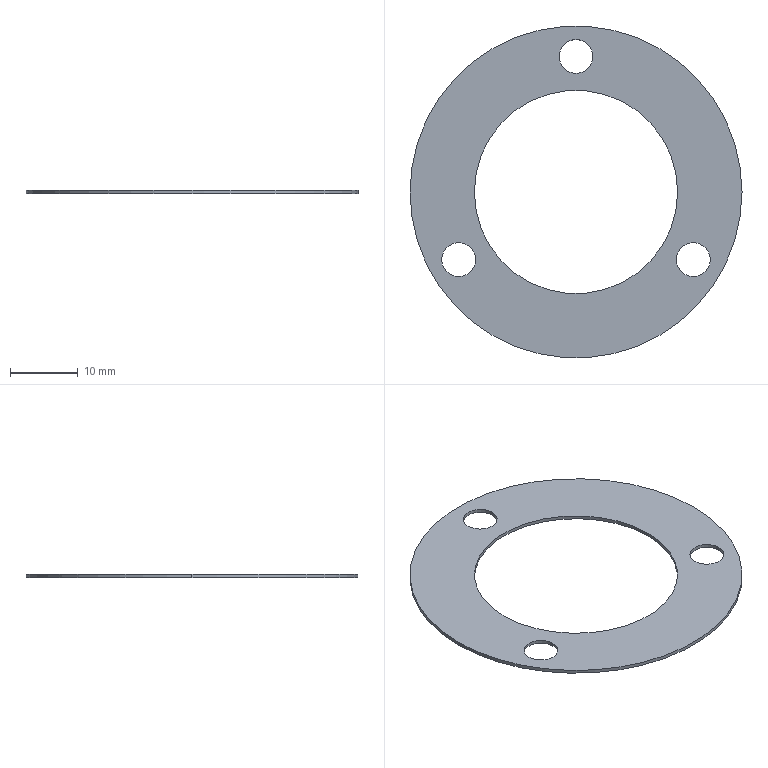Part | SolidWorks | features Extrusion 1, ICE 1 | 1 solid | 12 faces | box 49 x 49 x 0.5 mm | volume 559.989 mm3 | cylinder 10 | plane 2 | commonest cylinder face diameters 5 x6 30 x2 49 x2
STEP:
#1=CARTESIAN_POINT('',(-2.5,20.,0.));
#2=VERTEX_POINT('',#1);
#3=CARTESIAN_POINT('',(2.5,20.,0.));
#4=VERTEX_POINT('',#3);
#5=CARTESIAN_POINT('',(0.,20.,0.));
#6=DIRECTION('',(0.,0.,1.));
#7=DIRECTION('',(1.,0.,0.));
#8=AXIS2_PLACEMENT_3D('',#5,#6,#7);
#9=CIRCLE('',#8,2.5);
#10=EDGE_CURVE('',#2,#4,#9,.T.);
#11=ORIENTED_EDGE('',*,*,#10,.F.);
#12=CARTESIAN_POINT('',(-2.5,20.,0.5));
#13=VERTEX_POINT('',#12);
#14=CARTESIAN_POINT('',(-2.5,20.,0.));
#15=DIRECTION('',(0.,0.,1.));
#16=VECTOR('',#15,1000.);
#17=LINE('',#14,#16);
#18=EDGE_CURVE('',#2,#13,#17,.T.);
#19=ORIENTED_EDGE('',*,*,#18,.T.);
#20=CARTESIAN_POINT('',(2.5,20.,0.5));
#21=VERTEX_POINT('',#20);
#22=CARTESIAN_POINT('',(0.,20.,0.5));
#23=DIRECTION('',(0.,0.,1.));
#24=DIRECTION('',(1.,0.,0.));
#25=AXIS2_PLACEMENT_3D('',#22,#23,#24);
#26=CIRCLE('',#25,2.5);
#27=EDGE_CURVE('',#13,#21,#26,.T.);
#28=ORIENTED_EDGE('',*,*,#27,.T.);
#29=CARTESIAN_POINT('',(2.5,20.,0.));
#30=DIRECTION('',(0.,0.,1.));
#31=VECTOR('',#30,1000.);
#32=LINE('',#29,#31);
#33=EDGE_CURVE('',#4,#21,#32,.T.);
#34=ORIENTED_EDGE('',*,*,#33,.F.);
#35=EDGE_LOOP('',(#11,#19,#28,#34));
#36=FACE_OUTER_BOUND('',#35,.T.);
#37=CARTESIAN_POINT('',(0.,20.,0.));
#38=DIRECTION('',(0.,0.,1.));
#39=DIRECTION('',(1.,0.,0.));
#40=AXIS2_PLACEMENT_3D('',#37,#38,#39);
#41=CYLINDRICAL_SURFACE('',#40,2.5);
#42=ADVANCED_FACE('',(#36),#41,.F.);
#43=CARTESIAN_POINT('',(14.821,-10.,0.));
#44=VERTEX_POINT('',#43);
#45=CARTESIAN_POINT('',(19.821,-10.,0.));
#46=VERTEX_POINT('',#45);
#47=CARTESIAN_POINT('',(17.321,-10.,0.));
#48=DIRECTION('',(0.,0.,1.));
#49=DIRECTION('',(1.,0.,0.));
#50=AXIS2_PLACEMENT_3D('',#47,#48,#49);
#51=CIRCLE('',#50,2.5);
#52=EDGE_CURVE('',#44,#46,#51,.T.);
#53=ORIENTED_EDGE('',*,*,#52,.F.);
#54=CARTESIAN_POINT('',(14.821,-10.,0.5));
#55=VERTEX_POINT('',#54);
#56=CARTESIAN_POINT('',(14.821,-10.,0.));
#57=DIRECTION('',(0.,0.,1.));
#58=VECTOR('',#57,1000.);
#59=LINE('',#56,#58);
#60=EDGE_CURVE('',#44,#55,#59,.T.);
#61=ORIENTED_EDGE('',*,*,#60,.T.);
#62=CARTESIAN_POINT('',(19.821,-10.,0.5));
#63=VERTEX_POINT('',#62);
#64=CARTESIAN_POINT('',(17.321,-10.,0.5));
#65=DIRECTION('',(0.,0.,1.));
#66=DIRECTION('',(1.,0.,0.));
#67=AXIS2_PLACEMENT_3D('',#64,#65,#66);
#68=CIRCLE('',#67,2.5);
#69=EDGE_CURVE('',#55,#63,#68,.T.);
#70=ORIENTED_EDGE('',*,*,#69,.T.);
#71=CARTESIAN_POINT('',(19.821,-10.,0.));
#72=DIRECTION('',(0.,0.,1.));
#73=VECTOR('',#72,1000.);
#74=LINE('',#71,#73);
#75=EDGE_CURVE('',#46,#63,#74,.T.);
#76=ORIENTED_EDGE('',*,*,#75,.F.);
#77=EDGE_LOOP('',(#53,#61,#70,#76));
#78=FACE_OUTER_BOUND('',#77,.T.);
#79=CARTESIAN_POINT('',(17.321,-10.,0.));
#80=DIRECTION('',(0.,0.,1.));
#81=DIRECTION('',(1.,0.,0.));
#82=AXIS2_PLACEMENT_3D('',#79,#80,#81);
#83=CYLINDRICAL_SURFACE('',#82,2.5);
#84=ADVANCED_FACE('',(#78),#83,.F.);
#85=CARTESIAN_POINT('',(-19.821,-10.,0.));
#86=VERTEX_POINT('',#85);
#87=CARTESIAN_POINT('',(-14.821,-10.,0.));
#88=VERTEX_POINT('',#87);
#89=CARTESIAN_POINT('',(-17.321,-10.,0.));
#90=DIRECTION('',(0.,0.,1.));
#91=DIRECTION('',(1.,0.,0.));
#92=AXIS2_PLACEMENT_3D('',#89,#90,#91);
#93=CIRCLE('',#92,2.5);
#94=EDGE_CURVE('',#86,#88,#93,.T.);
#95=ORIENTED_EDGE('',*,*,#94,.F.);
#96=CARTESIAN_POINT('',(-19.821,-10.,0.5));
#97=VERTEX_POINT('',#96);
#98=CARTESIAN_POINT('',(-19.821,-10.,0.));
#99=DIRECTION('',(0.,0.,1.));
#100=VECTOR('',#99,1000.);
#101=LINE('',#98,#100);
#102=EDGE_CURVE('',#86,#97,#101,.T.);
#103=ORIENTED_EDGE('',*,*,#102,.T.);
#104=CARTESIAN_POINT('',(-14.821,-10.,0.5));
#105=VERTEX_POINT('',#104);
#106=CARTESIAN_POINT('',(-17.321,-10.,0.5));
#107=DIRECTION('',(0.,0.,1.));
#108=DIRECTION('',(1.,0.,0.));
#109=AXIS2_PLACEMENT_3D('',#106,#107,#108);
#110=CIRCLE('',#109,2.5);
#111=EDGE_CURVE('',#97,#105,#110,.T.);
#112=ORIENTED_EDGE('',*,*,#111,.T.);
#113=CARTESIAN_POINT('',(-14.821,-10.,0.));
#114=DIRECTION('',(0.,0.,1.));
#115=VECTOR('',#114,1000.);
#116=LINE('',#113,#115);
#117=EDGE_CURVE('',#88,#105,#116,.T.);
#118=ORIENTED_EDGE('',*,*,#117,.F.);
#119=EDGE_LOOP('',(#95,#103,#112,#118));
#120=FACE_OUTER_BOUND('',#119,.T.);
#121=CARTESIAN_POINT('',(-17.321,-10.,0.));
#122=DIRECTION('',(0.,0.,1.));
#123=DIRECTION('',(1.,0.,0.));
#124=AXIS2_PLACEMENT_3D('',#121,#122,#123);
#125=CYLINDRICAL_SURFACE('',#124,2.5);
#126=ADVANCED_FACE('',(#120),#125,.F.);
#127=CARTESIAN_POINT('',(-15.,0.,0.5));
#128=VERTEX_POINT('',#127);
#129=CARTESIAN_POINT('',(15.,0.,0.5));
#130=VERTEX_POINT('',#129);
#131=CARTESIAN_POINT('',(0.,0.,0.5));
#132=DIRECTION('',(0.,0.,1.));
#133=DIRECTION('',(1.,0.,0.));
#134=AXIS2_PLACEMENT_3D('',#131,#132,#133);
#135=CIRCLE('',#134,15.);
#136=EDGE_CURVE('',#128,#130,#135,.T.);
#137=ORIENTED_EDGE('',*,*,#136,.T.);
#138=CARTESIAN_POINT('',(15.,0.,0.));
#139=VERTEX_POINT('',#138);
#140=CARTESIAN_POINT('',(15.,0.,0.5));
#141=DIRECTION('',(0.,0.,-1.));
#142=VECTOR('',#141,1000.);
#143=LINE('',#140,#142);
#144=EDGE_CURVE('',#130,#139,#143,.T.);
#145=ORIENTED_EDGE('',*,*,#144,.T.);
#146=CARTESIAN_POINT('',(-15.,0.,0.));
#147=VERTEX_POINT('',#146);
#148=CARTESIAN_POINT('',(0.,0.,0.));
#149=DIRECTION('',(0.,0.,1.));
#150=DIRECTION('',(1.,0.,0.));
#151=AXIS2_PLACEMENT_3D('',#148,#149,#150);
#152=CIRCLE('',#151,15.);
#153=EDGE_CURVE('',#147,#139,#152,.T.);
#154=ORIENTED_EDGE('',*,*,#153,.F.);
#155=CARTESIAN_POINT('',(-15.,0.,0.5));
#156=DIRECTION('',(0.,0.,-1.));
#157=VECTOR('',#156,1000.);
#158=LINE('',#155,#157);
#159=EDGE_CURVE('',#128,#147,#158,.T.);
#160=ORIENTED_EDGE('',*,*,#159,.F.);
#161=EDGE_LOOP('',(#137,#145,#154,#160));
#162=FACE_OUTER_BOUND('',#161,.T.);
#163=CARTESIAN_POINT('',(0.,0.,0.5));
#164=DIRECTION('',(0.,0.,-1.));
#165=DIRECTION('',(-1.,0.,0.));
#166=AXIS2_PLACEMENT_3D('',#163,#164,#165);
#167=CYLINDRICAL_SURFACE('',#166,15.);
#168=ADVANCED_FACE('',(#162),#167,.F.);
#169=CARTESIAN_POINT('',(24.5,0.,0.5));
#170=VERTEX_POINT('',#169);
#171=CARTESIAN_POINT('',(-24.5,0.,0.5));
#172=VERTEX_POINT('',#171);
#173=CARTESIAN_POINT('',(0.,0.,0.5));
#174=DIRECTION('',(0.,0.,1.));
#175=DIRECTION('',(1.,0.,0.));
#176=AXIS2_PLACEMENT_3D('',#173,#174,#175);
#177=CIRCLE('',#176,24.5);
#178=EDGE_CURVE('',#170,#172,#177,.T.);
#179=ORIENTED_EDGE('',*,*,#178,.F.);
#180=CARTESIAN_POINT('',(24.5,0.,0.));
#181=VERTEX_POINT('',#180);
#182=CARTESIAN_POINT('',(24.5,0.,0.5));
#183=DIRECTION('',(0.,0.,-1.));
#184=VECTOR('',#183,1000.);
#185=LINE('',#182,#184);
#186=EDGE_CURVE('',#170,#181,#185,.T.);
#187=ORIENTED_EDGE('',*,*,#186,.T.);
#188=CARTESIAN_POINT('',(-24.5,0.,0.));
#189=VERTEX_POINT('',#188);
#190=CARTESIAN_POINT('',(0.,0.,0.));
#191=DIRECTION('',(0.,0.,1.));
#192=DIRECTION('',(1.,0.,0.));
#193=AXIS2_PLACEMENT_3D('',#190,#191,#192);
#194=CIRCLE('',#193,24.5);
#195=EDGE_CURVE('',#181,#189,#194,.T.);
#196=ORIENTED_EDGE('',*,*,#195,.T.);
#197=CARTESIAN_POINT('',(-24.5,0.,0.5));
#198=DIRECTION('',(0.,0.,-1.));
#199=VECTOR('',#198,1000.);
#200=LINE('',#197,#199);
#201=EDGE_CURVE('',#172,#189,#200,.T.);
#202=ORIENTED_EDGE('',*,*,#201,.F.);
#203=EDGE_LOOP('',(#179,#187,#196,#202));
#204=FACE_OUTER_BOUND('',#203,.T.);
#205=CARTESIAN_POINT('',(0.,0.,0.5));
#206=DIRECTION('',(0.,0.,-1.));
#207=DIRECTION('',(-1.,0.,0.));
#208=AXIS2_PLACEMENT_3D('',#205,#206,#207);
#209=CYLINDRICAL_SURFACE('',#208,24.5);
#210=ADVANCED_FACE('',(#204),#209,.T.);
#211=CARTESIAN_POINT('',(0.,20.,0.5));
#212=DIRECTION('',(0.,0.,1.));
#213=DIRECTION('',(1.,0.,0.));
#214=AXIS2_PLACEMENT_3D('',#211,#212,#213);
#215=CIRCLE('',#214,2.5);
#216=EDGE_CURVE('',#21,#13,#215,.T.);
#217=ORIENTED_EDGE('',*,*,#216,.F.);
#218=ORIENTED_EDGE('',*,*,#27,.F.);
#219=EDGE_LOOP('',(#217,#218));
#220=FACE_BOUND('',#219,.T.);
#221=CARTESIAN_POINT('',(17.321,-10.,0.5));
#222=DIRECTION('',(0.,0.,1.));
#223=DIRECTION('',(1.,0.,0.));
#224=AXIS2_PLACEMENT_3D('',#221,#222,#223);
#225=CIRCLE('',#224,2.5);
#226=EDGE_CURVE('',#63,#55,#225,.T.);
#227=ORIENTED_EDGE('',*,*,#226,.F.);
#228=ORIENTED_EDGE('',*,*,#69,.F.);
#229=EDGE_LOOP('',(#227,#228));
#230=FACE_BOUND('',#229,.T.);
#231=CARTESIAN_POINT('',(-17.321,-10.,0.5));
#232=DIRECTION('',(0.,0.,1.));
#233=DIRECTION('',(1.,0.,0.));
#234=AXIS2_PLACEMENT_3D('',#231,#232,#233);
#235=CIRCLE('',#234,2.5);
#236=EDGE_CURVE('',#105,#97,#235,.T.);
#237=ORIENTED_EDGE('',*,*,#236,.F.);
#238=ORIENTED_EDGE('',*,*,#111,.F.);
#239=EDGE_LOOP('',(#237,#238));
#240=FACE_BOUND('',#239,.T.);
#241=CARTESIAN_POINT('',(0.,0.,0.5));
#242=DIRECTION('',(0.,0.,1.));
#243=DIRECTION('',(1.,0.,0.));
#244=AXIS2_PLACEMENT_3D('',#241,#242,#243);
#245=CIRCLE('',#244,24.5);
#246=EDGE_CURVE('',#172,#170,#245,.T.);
#247=ORIENTED_EDGE('',*,*,#246,.T.);
#248=ORIENTED_EDGE('',*,*,#178,.T.);
#249=EDGE_LOOP('',(#247,#248));
#250=FACE_OUTER_BOUND('',#249,.T.);
#251=ORIENTED_EDGE('',*,*,#136,.F.);
#252=CARTESIAN_POINT('',(0.,0.,0.5));
#253=DIRECTION('',(0.,0.,1.));
#254=DIRECTION('',(1.,0.,0.));
#255=AXIS2_PLACEMENT_3D('',#252,#253,#254);
#256=CIRCLE('',#255,15.);
#257=EDGE_CURVE('',#130,#128,#256,.T.);
#258=ORIENTED_EDGE('',*,*,#257,.F.);
#259=EDGE_LOOP('',(#251,#258));
#260=FACE_BOUND('',#259,.T.);
#261=CARTESIAN_POINT('',(0.,0.,0.5));
#262=DIRECTION('',(0.,0.,1.));
#263=DIRECTION('',(1.,0.,0.));
#264=AXIS2_PLACEMENT_3D('',#261,#262,#263);
#265=PLANE('',#264);
#266=ADVANCED_FACE('',(#220,#230,#240,#250,#260),#265,.T.);
#267=CARTESIAN_POINT('',(0.,20.,0.));
#268=DIRECTION('',(0.,0.,1.));
#269=DIRECTION('',(1.,0.,0.));
#270=AXIS2_PLACEMENT_3D('',#267,#268,#269);
#271=CIRCLE('',#270,2.5);
#272=EDGE_CURVE('',#4,#2,#271,.T.);
#273=ORIENTED_EDGE('',*,*,#272,.T.);
#274=ORIENTED_EDGE('',*,*,#10,.T.);
#275=EDGE_LOOP('',(#273,#274));
#276=FACE_BOUND('',#275,.T.);
#277=CARTESIAN_POINT('',(17.321,-10.,0.));
#278=DIRECTION('',(0.,0.,1.));
#279=DIRECTION('',(1.,0.,0.));
#280=AXIS2_PLACEMENT_3D('',#277,#278,#279);
#281=CIRCLE('',#280,2.5);
#282=EDGE_CURVE('',#46,#44,#281,.T.);
#283=ORIENTED_EDGE('',*,*,#282,.T.);
#284=ORIENTED_EDGE('',*,*,#52,.T.);
#285=EDGE_LOOP('',(#283,#284));
#286=FACE_BOUND('',#285,.T.);
#287=CARTESIAN_POINT('',(-17.321,-10.,0.));
#288=DIRECTION('',(0.,0.,1.));
#289=DIRECTION('',(1.,0.,0.));
#290=AXIS2_PLACEMENT_3D('',#287,#288,#289);
#291=CIRCLE('',#290,2.5);
#292=EDGE_CURVE('',#88,#86,#291,.T.);
#293=ORIENTED_EDGE('',*,*,#292,.T.);
#294=ORIENTED_EDGE('',*,*,#94,.T.);
#295=EDGE_LOOP('',(#293,#294));
#296=FACE_BOUND('',#295,.T.);
#297=CARTESIAN_POINT('',(0.,0.,0.));
#298=DIRECTION('',(0.,0.,1.));
#299=DIRECTION('',(1.,0.,0.));
#300=AXIS2_PLACEMENT_3D('',#297,#298,#299);
#301=CIRCLE('',#300,24.5);
#302=EDGE_CURVE('',#189,#181,#301,.T.);
#303=ORIENTED_EDGE('',*,*,#302,.F.);
#304=ORIENTED_EDGE('',*,*,#195,.F.);
#305=EDGE_LOOP('',(#303,#304));
#306=FACE_OUTER_BOUND('',#305,.T.);
#307=ORIENTED_EDGE('',*,*,#153,.T.);
#308=CARTESIAN_POINT('',(0.,0.,0.));
#309=DIRECTION('',(0.,0.,1.));
#310=DIRECTION('',(1.,0.,0.));
#311=AXIS2_PLACEMENT_3D('',#308,#309,#310);
#312=CIRCLE('',#311,15.);
#313=EDGE_CURVE('',#139,#147,#312,.T.);
#314=ORIENTED_EDGE('',*,*,#313,.T.);
#315=EDGE_LOOP('',(#307,#314));
#316=FACE_BOUND('',#315,.T.);
#317=CARTESIAN_POINT('',(0.,0.,0.));
#318=DIRECTION('',(0.,0.,1.));
#319=DIRECTION('',(1.,0.,0.));
#320=AXIS2_PLACEMENT_3D('',#317,#318,#319);
#321=PLANE('',#320);
#322=ADVANCED_FACE('',(#276,#286,#296,#306,#316),#321,.F.);
#323=ORIENTED_EDGE('',*,*,#186,.F.);
#324=ORIENTED_EDGE('',*,*,#246,.F.);
#325=ORIENTED_EDGE('',*,*,#201,.T.);
#326=ORIENTED_EDGE('',*,*,#302,.T.);
#327=EDGE_LOOP('',(#323,#324,#325,#326));
#328=FACE_OUTER_BOUND('',#327,.T.);
#329=CARTESIAN_POINT('',(0.,0.,0.5));
#330=DIRECTION('',(0.,0.,-1.));
#331=DIRECTION('',(-1.,0.,0.));
#332=AXIS2_PLACEMENT_3D('',#329,#330,#331);
#333=CYLINDRICAL_SURFACE('',#332,24.5);
#334=ADVANCED_FACE('',(#328),#333,.T.);
#335=ORIENTED_EDGE('',*,*,#144,.F.);
#336=ORIENTED_EDGE('',*,*,#257,.T.);
#337=ORIENTED_EDGE('',*,*,#159,.T.);
#338=ORIENTED_EDGE('',*,*,#313,.F.);
#339=EDGE_LOOP('',(#335,#336,#337,#338));
#340=FACE_OUTER_BOUND('',#339,.T.);
#341=CARTESIAN_POINT('',(0.,0.,0.5));
#342=DIRECTION('',(0.,0.,-1.));
#343=DIRECTION('',(-1.,0.,0.));
#344=AXIS2_PLACEMENT_3D('',#341,#342,#343);
#345=CYLINDRICAL_SURFACE('',#344,15.);
#346=ADVANCED_FACE('',(#340),#345,.F.);
#347=ORIENTED_EDGE('',*,*,#102,.F.);
#348=ORIENTED_EDGE('',*,*,#292,.F.);
#349=ORIENTED_EDGE('',*,*,#117,.T.);
#350=ORIENTED_EDGE('',*,*,#236,.T.);
#351=EDGE_LOOP('',(#347,#348,#349,#350));
#352=FACE_OUTER_BOUND('',#351,.T.);
#353=CARTESIAN_POINT('',(-17.321,-10.,0.));
#354=DIRECTION('',(0.,0.,1.));
#355=DIRECTION('',(1.,0.,0.));
#356=AXIS2_PLACEMENT_3D('',#353,#354,#355);
#357=CYLINDRICAL_SURFACE('',#356,2.5);
#358=ADVANCED_FACE('',(#352),#357,.F.);
#359=ORIENTED_EDGE('',*,*,#60,.F.);
#360=ORIENTED_EDGE('',*,*,#282,.F.);
#361=ORIENTED_EDGE('',*,*,#75,.T.);
#362=ORIENTED_EDGE('',*,*,#226,.T.);
#363=EDGE_LOOP('',(#359,#360,#361,#362));
#364=FACE_OUTER_BOUND('',#363,.T.);
#365=CARTESIAN_POINT('',(17.321,-10.,0.));
#366=DIRECTION('',(0.,0.,1.));
#367=DIRECTION('',(1.,0.,0.));
#368=AXIS2_PLACEMENT_3D('',#365,#366,#367);
#369=CYLINDRICAL_SURFACE('',#368,2.5);
#370=ADVANCED_FACE('',(#364),#369,.F.);
#371=ORIENTED_EDGE('',*,*,#18,.F.);
#372=ORIENTED_EDGE('',*,*,#272,.F.);
#373=ORIENTED_EDGE('',*,*,#33,.T.);
#374=ORIENTED_EDGE('',*,*,#216,.T.);
#375=EDGE_LOOP('',(#371,#372,#373,#374));
#376=FACE_OUTER_BOUND('',#375,.T.);
#377=CARTESIAN_POINT('',(0.,20.,0.));
#378=DIRECTION('',(0.,0.,1.));
#379=DIRECTION('',(1.,0.,0.));
#380=AXIS2_PLACEMENT_3D('',#377,#378,#379);
#381=CYLINDRICAL_SURFACE('',#380,2.5);
#382=ADVANCED_FACE('',(#376),#381,.F.);
#383=CLOSED_SHELL('',(#42,#84,#126,#168,#210,#266,#322,#334,#346,#358,#370,#382));
#384=MANIFOLD_SOLID_BREP('',#383);
#385=CARTESIAN_POINT('',(0.,0.,0.));
#386=DIRECTION('',(0.,0.,1.));
#387=DIRECTION('',(1.,0.,0.));
#388=AXIS2_PLACEMENT_3D('',#385,#386,#387);
#389=(LENGTH_UNIT()NAMED_UNIT(*)SI_UNIT(.MILLI.,.METRE.));
#390=UNCERTAINTY_MEASURE_WITH_UNIT(LENGTH_MEASURE(0.00001),#389,'','');
#391=(NAMED_UNIT(*)PLANE_ANGLE_UNIT()SI_UNIT($,.RADIAN.));
#392=(NAMED_UNIT(*)SI_UNIT($,.STERADIAN.)SOLID_ANGLE_UNIT());
#393=(GEOMETRIC_REPRESENTATION_CONTEXT(3)GLOBAL_UNCERTAINTY_ASSIGNED_CONTEXT((#390))GLOBAL_UNIT_ASSIGNED_CONTEXT((#389,#391,#392))REPRESENTATION_CONTEXT('',''));
#394=ADVANCED_BREP_SHAPE_REPRESENTATION('',(#384,#388),#393);